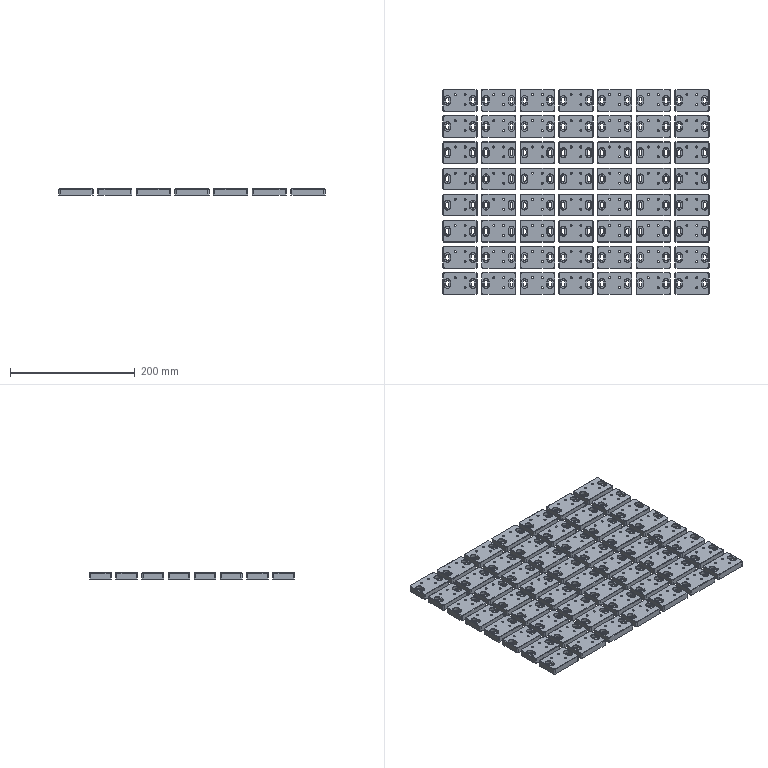Part | 56 solids | 2800 faces | box 427 x 329 x 10 mm | volume 968173 mm3 | plane 1344 | cylinder 1008 | cone 448 | commonest cylinder face diameters 3.3 x336 4 x224 4.5 x224 9.5 x224